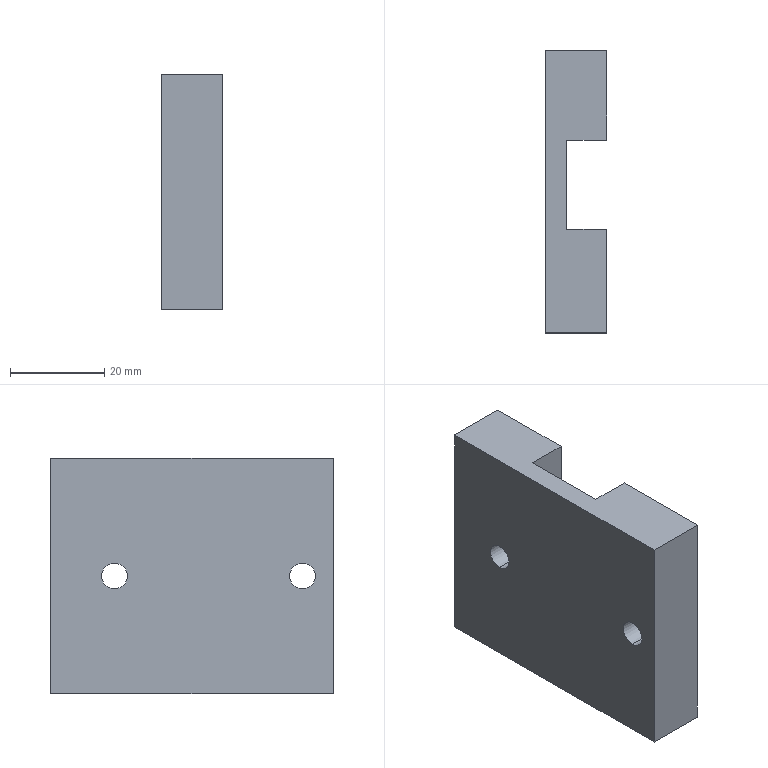Part | STEP file | PN_0039 | 1 solid | 20 faces | box 13 x 60 x 50 mm | volume 29683 mm3 | plane 12 | cylinder 8 | commonest cylinder face diameters 5.5 x4 10 x4
STEP:
#1=CARTESIAN_POINT('',(0.,0.,0.));
#2=DIRECTION('',(0.,0.,1.));
#3=DIRECTION('',(1.,0.,0.));
#4=AXIS2_PLACEMENT_3D('',#1,#2,#3);
#5=CARTESIAN_POINT('',(19.5,80.,-2.75));
#6=VERTEX_POINT('',#5);
#7=CARTESIAN_POINT('',(26.8,80.,-2.75));
#8=VERTEX_POINT('',#7);
#9=CARTESIAN_POINT('',(23.4,80.,-2.75));
#10=DIRECTION('',(1.,0.,0.));
#11=VECTOR('',#10,1.);
#12=LINE('',#9,#11);
#13=CARTESIAN_POINT('',(23.4,80.,0.));
#14=DIRECTION('',(1.,0.,0.));
#15=DIRECTION('',(0.,0.,-1.));
#16=AXIS2_PLACEMENT_3D('',#13,#14,#15);
#17=CYLINDRICAL_SURFACE('',#16,2.75);
#18=CARTESIAN_POINT('',(6.283,0.));
#19=DIRECTION('',(0.,1.));
#20=VECTOR('',#19,1.);
#21=LINE('',#18,#20);
#22=(GEOMETRIC_REPRESENTATION_CONTEXT(2)PARAMETRIC_REPRESENTATION_CONTEXT()REPRESENTATION_CONTEXT('',''));
#23=DEFINITIONAL_REPRESENTATION('',(#21),#22);
#24=PCURVE('',#17,#23);
#25=CARTESIAN_POINT('',(23.4,80.,0.));
#26=DIRECTION('',(1.,0.,0.));
#27=DIRECTION('',(0.,0.,-1.));
#28=AXIS2_PLACEMENT_3D('',#25,#26,#27);
#29=CYLINDRICAL_SURFACE('',#28,2.75);
#30=CARTESIAN_POINT('',(0.,0.));
#31=DIRECTION('',(0.,1.));
#32=VECTOR('',#31,1.);
#33=LINE('',#30,#32);
#34=(GEOMETRIC_REPRESENTATION_CONTEXT(2)PARAMETRIC_REPRESENTATION_CONTEXT()REPRESENTATION_CONTEXT('',''));
#35=DEFINITIONAL_REPRESENTATION('',(#33),#34);
#36=PCURVE('',#29,#35);
#37=SURFACE_CURVE('',#12,(#24,#36),.PCURVE_S1.);
#38=EDGE_CURVE('',#6,#8,#37,.T.);
#39=ORIENTED_EDGE('',*,*,#38,.T.);
#40=CARTESIAN_POINT('',(26.8,80.,2.75));
#41=VERTEX_POINT('',#40);
#42=CARTESIAN_POINT('',(26.8,80.,0.));
#43=DIRECTION('',(-1.,0.,0.));
#44=DIRECTION('',(0.,0.,-1.));
#45=AXIS2_PLACEMENT_3D('',#42,#43,#44);
#46=CIRCLE('',#45,2.75);
#47=CARTESIAN_POINT('',(6.283,3.4));
#48=DIRECTION('',(-1.,0.));
#49=VECTOR('',#48,1.);
#50=LINE('',#47,#49);
#51=(GEOMETRIC_REPRESENTATION_CONTEXT(2)PARAMETRIC_REPRESENTATION_CONTEXT()REPRESENTATION_CONTEXT('',''));
#52=DEFINITIONAL_REPRESENTATION('',(#50),#51);
#53=PCURVE('',#17,#52);
#54=CARTESIAN_POINT('',(26.8,83.875,0.));
#55=DIRECTION('',(-1.,0.,0.));
#56=DIRECTION('',(0.,0.,1.));
#57=AXIS2_PLACEMENT_3D('',#54,#55,#56);
#58=PLANE('',#57);
#59=CARTESIAN_POINT('',(0.,-3.875));
#60=DIRECTION('',(-1.,0.));
#61=AXIS2_PLACEMENT_2D('',#59,#60);
#62=CIRCLE('',#61,2.75);
#63=(GEOMETRIC_REPRESENTATION_CONTEXT(2)PARAMETRIC_REPRESENTATION_CONTEXT()REPRESENTATION_CONTEXT('',''));
#64=DEFINITIONAL_REPRESENTATION('',(#62),#63);
#65=PCURVE('',#58,#64);
#66=SURFACE_CURVE('',#46,(#53,#65),.PCURVE_S1.);
#67=EDGE_CURVE('',#8,#41,#66,.T.);
#68=ORIENTED_EDGE('',*,*,#67,.T.);
#69=CARTESIAN_POINT('',(19.5,80.,2.75));
#70=VERTEX_POINT('',#69);
#71=CARTESIAN_POINT('',(23.4,80.,2.75));
#72=DIRECTION('',(1.,0.,0.));
#73=VECTOR('',#72,1.);
#74=LINE('',#71,#73);
#75=CARTESIAN_POINT('',(3.142,0.));
#76=DIRECTION('',(0.,1.));
#77=VECTOR('',#76,1.);
#78=LINE('',#75,#77);
#79=(GEOMETRIC_REPRESENTATION_CONTEXT(2)PARAMETRIC_REPRESENTATION_CONTEXT()REPRESENTATION_CONTEXT('',''));
#80=DEFINITIONAL_REPRESENTATION('',(#78),#79);
#81=PCURVE('',#17,#80);
#82=CARTESIAN_POINT('',(3.142,0.));
#83=DIRECTION('',(0.,1.));
#84=VECTOR('',#83,1.);
#85=LINE('',#82,#84);
#86=(GEOMETRIC_REPRESENTATION_CONTEXT(2)PARAMETRIC_REPRESENTATION_CONTEXT()REPRESENTATION_CONTEXT('',''));
#87=DEFINITIONAL_REPRESENTATION('',(#85),#86);
#88=PCURVE('',#29,#87);
#89=SURFACE_CURVE('',#74,(#81,#88),.PCURVE_S1.);
#90=EDGE_CURVE('',#70,#41,#89,.T.);
#91=ORIENTED_EDGE('',*,*,#90,.F.);
#92=CARTESIAN_POINT('',(19.5,80.,0.));
#93=DIRECTION('',(-1.,0.,0.));
#94=DIRECTION('',(0.,0.,1.));
#95=AXIS2_PLACEMENT_3D('',#92,#93,#94);
#96=CIRCLE('',#95,2.75);
#97=CARTESIAN_POINT('',(9.425,-3.9));
#98=DIRECTION('',(-1.,0.));
#99=VECTOR('',#98,1.);
#100=LINE('',#97,#99);
#101=(GEOMETRIC_REPRESENTATION_CONTEXT(2)PARAMETRIC_REPRESENTATION_CONTEXT()REPRESENTATION_CONTEXT('',''));
#102=DEFINITIONAL_REPRESENTATION('',(#100),#101);
#103=PCURVE('',#17,#102);
#104=CARTESIAN_POINT('',(19.5,33.5,-25.));
#105=DIRECTION('',(-1.,0.,0.));
#106=DIRECTION('',(0.,0.,1.));
#107=AXIS2_PLACEMENT_3D('',#104,#105,#106);
#108=PLANE('',#107);
#109=CARTESIAN_POINT('',(25.,46.5));
#110=DIRECTION('',(1.,0.));
#111=AXIS2_PLACEMENT_2D('',#109,#110);
#112=CIRCLE('',#111,2.75);
#113=(GEOMETRIC_REPRESENTATION_CONTEXT(2)PARAMETRIC_REPRESENTATION_CONTEXT()REPRESENTATION_CONTEXT('',''));
#114=DEFINITIONAL_REPRESENTATION('',(#112),#113);
#115=PCURVE('',#108,#114);
#116=SURFACE_CURVE('',#96,(#103,#115),.PCURVE_S1.);
#117=EDGE_CURVE('',#6,#70,#116,.T.);
#118=ORIENTED_EDGE('',*,*,#117,.F.);
#119=EDGE_LOOP('',(#39,#68,#91,#118));
#120=FACE_BOUND('',#119,.F.);
#121=ADVANCED_FACE('',(#120),#17,.F.);
#122=CARTESIAN_POINT('',(19.5,40.,-2.75));
#123=VERTEX_POINT('',#122);
#124=CARTESIAN_POINT('',(26.8,40.,-2.75));
#125=VERTEX_POINT('',#124);
#126=CARTESIAN_POINT('',(23.4,40.,-2.75));
#127=DIRECTION('',(1.,0.,0.));
#128=VECTOR('',#127,1.);
#129=LINE('',#126,#128);
#130=CARTESIAN_POINT('',(23.4,40.,0.));
#131=DIRECTION('',(1.,0.,0.));
#132=DIRECTION('',(0.,0.,-1.));
#133=AXIS2_PLACEMENT_3D('',#130,#131,#132);
#134=CYLINDRICAL_SURFACE('',#133,2.75);
#135=CARTESIAN_POINT('',(6.283,0.));
#136=DIRECTION('',(0.,1.));
#137=VECTOR('',#136,1.);
#138=LINE('',#135,#137);
#139=(GEOMETRIC_REPRESENTATION_CONTEXT(2)PARAMETRIC_REPRESENTATION_CONTEXT()REPRESENTATION_CONTEXT('',''));
#140=DEFINITIONAL_REPRESENTATION('',(#138),#139);
#141=PCURVE('',#134,#140);
#142=CARTESIAN_POINT('',(23.4,40.,0.));
#143=DIRECTION('',(1.,0.,0.));
#144=DIRECTION('',(0.,0.,-1.));
#145=AXIS2_PLACEMENT_3D('',#142,#143,#144);
#146=CYLINDRICAL_SURFACE('',#145,2.75);
#147=CARTESIAN_POINT('',(0.,0.));
#148=DIRECTION('',(0.,1.));
#149=VECTOR('',#148,1.);
#150=LINE('',#147,#149);
#151=(GEOMETRIC_REPRESENTATION_CONTEXT(2)PARAMETRIC_REPRESENTATION_CONTEXT()REPRESENTATION_CONTEXT('',''));
#152=DEFINITIONAL_REPRESENTATION('',(#150),#151);
#153=PCURVE('',#146,#152);
#154=SURFACE_CURVE('',#129,(#141,#153),.PCURVE_S1.);
#155=EDGE_CURVE('',#123,#125,#154,.T.);
#156=ORIENTED_EDGE('',*,*,#155,.T.);
#157=CARTESIAN_POINT('',(26.8,40.,2.75));
#158=VERTEX_POINT('',#157);
#159=CARTESIAN_POINT('',(26.8,40.,0.));
#160=DIRECTION('',(-1.,0.,0.));
#161=DIRECTION('',(0.,0.,-1.));
#162=AXIS2_PLACEMENT_3D('',#159,#160,#161);
#163=CIRCLE('',#162,2.75);
#164=CARTESIAN_POINT('',(6.283,3.4));
#165=DIRECTION('',(-1.,0.));
#166=VECTOR('',#165,1.);
#167=LINE('',#164,#166);
#168=(GEOMETRIC_REPRESENTATION_CONTEXT(2)PARAMETRIC_REPRESENTATION_CONTEXT()REPRESENTATION_CONTEXT('',''));
#169=DEFINITIONAL_REPRESENTATION('',(#167),#168);
#170=PCURVE('',#134,#169);
#171=CARTESIAN_POINT('',(26.8,43.875,0.));
#172=DIRECTION('',(-1.,0.,0.));
#173=DIRECTION('',(0.,0.,1.));
#174=AXIS2_PLACEMENT_3D('',#171,#172,#173);
#175=PLANE('',#174);
#176=CARTESIAN_POINT('',(0.,-3.875));
#177=DIRECTION('',(-1.,0.));
#178=AXIS2_PLACEMENT_2D('',#176,#177);
#179=CIRCLE('',#178,2.75);
#180=(GEOMETRIC_REPRESENTATION_CONTEXT(2)PARAMETRIC_REPRESENTATION_CONTEXT()REPRESENTATION_CONTEXT('',''));
#181=DEFINITIONAL_REPRESENTATION('',(#179),#180);
#182=PCURVE('',#175,#181);
#183=SURFACE_CURVE('',#163,(#170,#182),.PCURVE_S1.);
#184=EDGE_CURVE('',#125,#158,#183,.T.);
#185=ORIENTED_EDGE('',*,*,#184,.T.);
#186=CARTESIAN_POINT('',(19.5,40.,2.75));
#187=VERTEX_POINT('',#186);
#188=CARTESIAN_POINT('',(23.4,40.,2.75));
#189=DIRECTION('',(1.,0.,0.));
#190=VECTOR('',#189,1.);
#191=LINE('',#188,#190);
#192=CARTESIAN_POINT('',(3.142,0.));
#193=DIRECTION('',(0.,1.));
#194=VECTOR('',#193,1.);
#195=LINE('',#192,#194);
#196=(GEOMETRIC_REPRESENTATION_CONTEXT(2)PARAMETRIC_REPRESENTATION_CONTEXT()REPRESENTATION_CONTEXT('',''));
#197=DEFINITIONAL_REPRESENTATION('',(#195),#196);
#198=PCURVE('',#134,#197);
#199=CARTESIAN_POINT('',(3.142,0.));
#200=DIRECTION('',(0.,1.));
#201=VECTOR('',#200,1.);
#202=LINE('',#199,#201);
#203=(GEOMETRIC_REPRESENTATION_CONTEXT(2)PARAMETRIC_REPRESENTATION_CONTEXT()REPRESENTATION_CONTEXT('',''));
#204=DEFINITIONAL_REPRESENTATION('',(#202),#203);
#205=PCURVE('',#146,#204);
#206=SURFACE_CURVE('',#191,(#198,#205),.PCURVE_S1.);
#207=EDGE_CURVE('',#187,#158,#206,.T.);
#208=ORIENTED_EDGE('',*,*,#207,.F.);
#209=CARTESIAN_POINT('',(19.5,40.,0.));
#210=DIRECTION('',(-1.,0.,0.));
#211=DIRECTION('',(0.,0.,1.));
#212=AXIS2_PLACEMENT_3D('',#209,#210,#211);
#213=CIRCLE('',#212,2.75);
#214=CARTESIAN_POINT('',(9.425,-3.9));
#215=DIRECTION('',(-1.,0.));
#216=VECTOR('',#215,1.);
#217=LINE('',#214,#216);
#218=(GEOMETRIC_REPRESENTATION_CONTEXT(2)PARAMETRIC_REPRESENTATION_CONTEXT()REPRESENTATION_CONTEXT('',''));
#219=DEFINITIONAL_REPRESENTATION('',(#217),#218);
#220=PCURVE('',#134,#219);
#221=CARTESIAN_POINT('',(25.,6.5));
#222=DIRECTION('',(1.,0.));
#223=AXIS2_PLACEMENT_2D('',#221,#222);
#224=CIRCLE('',#223,2.75);
#225=(GEOMETRIC_REPRESENTATION_CONTEXT(2)PARAMETRIC_REPRESENTATION_CONTEXT()REPRESENTATION_CONTEXT('',''));
#226=DEFINITIONAL_REPRESENTATION('',(#224),#225);
#227=PCURVE('',#108,#226);
#228=SURFACE_CURVE('',#213,(#220,#227),.PCURVE_S1.);
#229=EDGE_CURVE('',#123,#187,#228,.T.);
#230=ORIENTED_EDGE('',*,*,#229,.F.);
#231=EDGE_LOOP('',(#156,#185,#208,#230));
#232=FACE_BOUND('',#231,.F.);
#233=ADVANCED_FACE('',(#232),#134,.F.);
#234=CARTESIAN_POINT('',(26.8,80.,-5.));
#235=VERTEX_POINT('',#234);
#236=CARTESIAN_POINT('',(32.5,80.,-5.));
#237=VERTEX_POINT('',#236);
#238=CARTESIAN_POINT('',(29.65,80.,-5.));
#239=DIRECTION('',(1.,0.,0.));
#240=VECTOR('',#239,1.);
#241=LINE('',#238,#240);
#242=CARTESIAN_POINT('',(29.65,80.,0.));
#243=DIRECTION('',(1.,0.,0.));
#244=DIRECTION('',(0.,0.,-1.));
#245=AXIS2_PLACEMENT_3D('',#242,#243,#244);
#246=CYLINDRICAL_SURFACE('',#245,5.);
#247=CARTESIAN_POINT('',(6.283,0.));
#248=DIRECTION('',(0.,1.));
#249=VECTOR('',#248,1.);
#250=LINE('',#247,#249);
#251=(GEOMETRIC_REPRESENTATION_CONTEXT(2)PARAMETRIC_REPRESENTATION_CONTEXT()REPRESENTATION_CONTEXT('',''));
#252=DEFINITIONAL_REPRESENTATION('',(#250),#251);
#253=PCURVE('',#246,#252);
#254=CARTESIAN_POINT('',(29.65,80.,0.));
#255=DIRECTION('',(1.,0.,0.));
#256=DIRECTION('',(0.,0.,-1.));
#257=AXIS2_PLACEMENT_3D('',#254,#255,#256);
#258=CYLINDRICAL_SURFACE('',#257,5.);
#259=CARTESIAN_POINT('',(0.,0.));
#260=DIRECTION('',(0.,1.));
#261=VECTOR('',#260,1.);
#262=LINE('',#259,#261);
#263=(GEOMETRIC_REPRESENTATION_CONTEXT(2)PARAMETRIC_REPRESENTATION_CONTEXT()REPRESENTATION_CONTEXT('',''));
#264=DEFINITIONAL_REPRESENTATION('',(#262),#263);
#265=PCURVE('',#258,#264);
#266=SURFACE_CURVE('',#241,(#253,#265),.PCURVE_S1.);
#267=EDGE_CURVE('',#235,#237,#266,.T.);
#268=ORIENTED_EDGE('',*,*,#267,.T.);
#269=CARTESIAN_POINT('',(32.5,80.,5.));
#270=VERTEX_POINT('',#269);
#271=CARTESIAN_POINT('',(32.5,80.,0.));
#272=DIRECTION('',(-1.,0.,0.));
#273=DIRECTION('',(0.,0.,-1.));
#274=AXIS2_PLACEMENT_3D('',#271,#272,#273);
#275=CIRCLE('',#274,5.);
#276=CARTESIAN_POINT('',(6.283,2.85));
#277=DIRECTION('',(-1.,0.));
#278=VECTOR('',#277,1.);
#279=LINE('',#276,#278);
#280=(GEOMETRIC_REPRESENTATION_CONTEXT(2)PARAMETRIC_REPRESENTATION_CONTEXT()REPRESENTATION_CONTEXT('',''));
#281=DEFINITIONAL_REPRESENTATION('',(#279),#280);
#282=PCURVE('',#246,#281);
#283=CARTESIAN_POINT('',(32.5,74.5,25.));
#284=DIRECTION('',(1.,0.,0.));
#285=DIRECTION('',(0.,0.,-1.));
#286=AXIS2_PLACEMENT_3D('',#283,#284,#285);
#287=PLANE('',#286);
#288=CARTESIAN_POINT('',(30.,5.5));
#289=CARTESIAN_POINT('',(30.,-3.16));
#290=CARTESIAN_POINT('',(22.5,1.17));
#291=CARTESIAN_POINT('',(15.,5.5));
#292=CARTESIAN_POINT('',(22.5,9.83));
#293=CARTESIAN_POINT('',(30.,14.16));
#294=CARTESIAN_POINT('',(30.,5.5));
#295=(BOUNDED_CURVE()B_SPLINE_CURVE(2,(#288,#289,#290,#291,#292,#293,#294),.UNSPECIFIED.,.T.,.F.)B_SPLINE_CURVE_WITH_KNOTS((1,2,2,2,2,1),(-2.094,0.,2.094,4.189,6.283,8.378),.UNSPECIFIED.)CURVE()GEOMETRIC_REPRESENTATION_ITEM()RATIONAL_B_SPLINE_CURVE((1.,0.5,1.,0.5,1.,0.5,1.))REPRESENTATION_ITEM(''));
#296=(GEOMETRIC_REPRESENTATION_CONTEXT(2)PARAMETRIC_REPRESENTATION_CONTEXT()REPRESENTATION_CONTEXT('',''));
#297=DEFINITIONAL_REPRESENTATION('',(#295),#296);
#298=PCURVE('',#287,#297);
#299=SURFACE_CURVE('',#275,(#282,#298),.PCURVE_S1.);
#300=EDGE_CURVE('',#237,#270,#299,.T.);
#301=ORIENTED_EDGE('',*,*,#300,.T.);
#302=CARTESIAN_POINT('',(26.8,80.,5.));
#303=VERTEX_POINT('',#302);
#304=CARTESIAN_POINT('',(29.65,80.,5.));
#305=DIRECTION('',(1.,0.,0.));
#306=VECTOR('',#305,1.);
#307=LINE('',#304,#306);
#308=CARTESIAN_POINT('',(3.142,0.));
#309=DIRECTION('',(0.,1.));
#310=VECTOR('',#309,1.);
#311=LINE('',#308,#310);
#312=(GEOMETRIC_REPRESENTATION_CONTEXT(2)PARAMETRIC_REPRESENTATION_CONTEXT()REPRESENTATION_CONTEXT('',''));
#313=DEFINITIONAL_REPRESENTATION('',(#311),#312);
#314=PCURVE('',#246,#313);
#315=CARTESIAN_POINT('',(3.142,0.));
#316=DIRECTION('',(0.,1.));
#317=VECTOR('',#316,1.);
#318=LINE('',#315,#317);
#319=(GEOMETRIC_REPRESENTATION_CONTEXT(2)PARAMETRIC_REPRESENTATION_CONTEXT()REPRESENTATION_CONTEXT('',''));
#320=DEFINITIONAL_REPRESENTATION('',(#318),#319);
#321=PCURVE('',#258,#320);
#322=SURFACE_CURVE('',#307,(#314,#321),.PCURVE_S1.);
#323=EDGE_CURVE('',#303,#270,#322,.T.);
#324=ORIENTED_EDGE('',*,*,#323,.F.);
#325=CARTESIAN_POINT('',(26.8,80.,0.));
#326=DIRECTION('',(-1.,0.,0.));
#327=DIRECTION('',(0.,0.,-1.));
#328=AXIS2_PLACEMENT_3D('',#325,#326,#327);
#329=CIRCLE('',#328,5.);
#330=CARTESIAN_POINT('',(6.283,-2.85));
#331=DIRECTION('',(-1.,0.));
#332=VECTOR('',#331,1.);
#333=LINE('',#330,#332);
#334=(GEOMETRIC_REPRESENTATION_CONTEXT(2)PARAMETRIC_REPRESENTATION_CONTEXT()REPRESENTATION_CONTEXT('',''));
#335=DEFINITIONAL_REPRESENTATION('',(#333),#334);
#336=PCURVE('',#246,#335);
#337=CARTESIAN_POINT('',(0.,-3.875));
#338=DIRECTION('',(-1.,0.));
#339=AXIS2_PLACEMENT_2D('',#337,#338);
#340=CIRCLE('',#339,5.);
#341=(GEOMETRIC_REPRESENTATION_CONTEXT(2)PARAMETRIC_REPRESENTATION_CONTEXT()REPRESENTATION_CONTEXT('',''));
#342=DEFINITIONAL_REPRESENTATION('',(#340),#341);
#343=PCURVE('',#58,#342);
#344=SURFACE_CURVE('',#329,(#336,#343),.PCURVE_S1.);
#345=EDGE_CURVE('',#235,#303,#344,.T.);
#346=ORIENTED_EDGE('',*,*,#345,.F.);
#347=EDGE_LOOP('',(#268,#301,#324,#346));
#348=FACE_BOUND('',#347,.F.);
#349=ADVANCED_FACE('',(#348),#246,.F.);
#350=CARTESIAN_POINT('',(26.8,40.,-5.));
#351=VERTEX_POINT('',#350);
#352=CARTESIAN_POINT('',(32.5,40.,-5.));
#353=VERTEX_POINT('',#352);
#354=CARTESIAN_POINT('',(29.65,40.,-5.));
#355=DIRECTION('',(1.,0.,0.));
#356=VECTOR('',#355,1.);
#357=LINE('',#354,#356);
#358=CARTESIAN_POINT('',(29.65,40.,0.));
#359=DIRECTION('',(1.,0.,0.));
#360=DIRECTION('',(0.,0.,-1.));
#361=AXIS2_PLACEMENT_3D('',#358,#359,#360);
#362=CYLINDRICAL_SURFACE('',#361,5.);
#363=CARTESIAN_POINT('',(6.283,0.));
#364=DIRECTION('',(0.,1.));
#365=VECTOR('',#364,1.);
#366=LINE('',#363,#365);
#367=(GEOMETRIC_REPRESENTATION_CONTEXT(2)PARAMETRIC_REPRESENTATION_CONTEXT()REPRESENTATION_CONTEXT('',''));
#368=DEFINITIONAL_REPRESENTATION('',(#366),#367);
#369=PCURVE('',#362,#368);
#370=CARTESIAN_POINT('',(29.65,40.,0.));
#371=DIRECTION('',(1.,0.,0.));
#372=DIRECTION('',(0.,0.,-1.));
#373=AXIS2_PLACEMENT_3D('',#370,#371,#372);
#374=CYLINDRICAL_SURFACE('',#373,5.);
#375=CARTESIAN_POINT('',(0.,0.));
#376=DIRECTION('',(0.,1.));
#377=VECTOR('',#376,1.);
#378=LINE('',#375,#377);
#379=(GEOMETRIC_REPRESENTATION_CONTEXT(2)PARAMETRIC_REPRESENTATION_CONTEXT()REPRESENTATION_CONTEXT('',''));
#380=DEFINITIONAL_REPRESENTATION('',(#378),#379);
#381=PCURVE('',#374,#380);
#382=SURFACE_CURVE('',#357,(#369,#381),.PCURVE_S1.);
#383=EDGE_CURVE('',#351,#353,#382,.T.);
#384=ORIENTED_EDGE('',*,*,#383,.T.);
#385=CARTESIAN_POINT('',(32.5,40.,5.));
#386=VERTEX_POINT('',#385);
#387=CARTESIAN_POINT('',(32.5,40.,0.));
#388=DIRECTION('',(-1.,0.,0.));
#389=DIRECTION('',(0.,0.,-1.));
#390=AXIS2_PLACEMENT_3D('',#387,#388,#389);
#391=CIRCLE('',#390,5.);
#392=CARTESIAN_POINT('',(6.283,2.85));
#393=DIRECTION('',(-1.,0.));
#394=VECTOR('',#393,1.);
#395=LINE('',#392,#394);
#396=(GEOMETRIC_REPRESENTATION_CONTEXT(2)PARAMETRIC_REPRESENTATION_CONTEXT()REPRESENTATION_CONTEXT('',''));
#397=DEFINITIONAL_REPRESENTATION('',(#395),#396);
#398=PCURVE('',#362,#397);
#399=CARTESIAN_POINT('',(32.5,33.5,25.));
#400=DIRECTION('',(1.,0.,0.));
#401=DIRECTION('',(0.,0.,-1.));
#402=AXIS2_PLACEMENT_3D('',#399,#400,#401);
#403=PLANE('',#402);
#404=CARTESIAN_POINT('',(30.,6.5));
#405=CARTESIAN_POINT('',(30.,-2.16));
#406=CARTESIAN_POINT('',(22.5,2.17));
#407=CARTESIAN_POINT('',(15.,6.5));
#408=CARTESIAN_POINT('',(22.5,10.83));
#409=CARTESIAN_POINT('',(30.,15.16));
#410=CARTESIAN_POINT('',(30.,6.5));
#411=(BOUNDED_CURVE()B_SPLINE_CURVE(2,(#404,#405,#406,#407,#408,#409,#410),.UNSPECIFIED.,.T.,.F.)B_SPLINE_CURVE_WITH_KNOTS((1,2,2,2,2,1),(-2.094,0.,2.094,4.189,6.283,8.378),.UNSPECIFIED.)CURVE()GEOMETRIC_REPRESENTATION_ITEM()RATIONAL_B_SPLINE_CURVE((1.,0.5,1.,0.5,1.,0.5,1.))REPRESENTATION_ITEM(''));
#412=(GEOMETRIC_REPRESENTATION_CONTEXT(2)PARAMETRIC_REPRESENTATION_CONTEXT()REPRESENTATION_CONTEXT('',''));
#413=DEFINITIONAL_REPRESENTATION('',(#411),#412);
#414=PCURVE('',#403,#413);
#415=SURFACE_CURVE('',#391,(#398,#414),.PCURVE_S1.);
#416=EDGE_CURVE('',#353,#386,#415,.T.);
#417=ORIENTED_EDGE('',*,*,#416,.T.);
#418=CARTESIAN_POINT('',(26.8,40.,5.));
#419=VERTEX_POINT('',#418);
#420=CARTESIAN_POINT('',(29.65,40.,5.));
#421=DIRECTION('',(1.,0.,0.));
#422=VECTOR('',#421,1.);
#423=LINE('',#420,#422);
#424=CARTESIAN_POINT('',(3.142,0.));
#425=DIRECTION('',(0.,1.));
#426=VECTOR('',#425,1.);
#427=LINE('',#424,#426);
#428=(GEOMETRIC_REPRESENTATION_CONTEXT(2)PARAMETRIC_REPRESENTATION_CONTEXT()REPRESENTATION_CONTEXT('',''));
#429=DEFINITIONAL_REPRESENTATION('',(#427),#428);
#430=PCURVE('',#362,#429);
#431=CARTESIAN_POINT('',(3.142,0.));
#432=DIRECTION('',(0.,1.));
#433=VECTOR('',#432,1.);
#434=LINE('',#431,#433);
#435=(GEOMETRIC_REPRESENTATION_CONTEXT(2)PARAMETRIC_REPRESENTATION_CONTEXT()REPRESENTATION_CONTEXT('',''));
#436=DEFINITIONAL_REPRESENTATION('',(#434),#435);
#437=PCURVE('',#374,#436);
#438=SURFACE_CURVE('',#423,(#430,#437),.PCURVE_S1.);
#439=EDGE_CURVE('',#419,#386,#438,.T.);
#440=ORIENTED_EDGE('',*,*,#439,.F.);
#441=CARTESIAN_POINT('',(26.8,40.,0.));
#442=DIRECTION('',(-1.,0.,0.));
#443=DIRECTION('',(0.,0.,-1.));
#444=AXIS2_PLACEMENT_3D('',#441,#442,#443);
#445=CIRCLE('',#444,5.);
#446=CARTESIAN_POINT('',(6.283,-2.85));
#447=DIRECTION('',(-1.,0.));
#448=VECTOR('',#447,1.);
#449=LINE('',#446,#448);
#450=(GEOMETRIC_REPRESENTATION_CONTEXT(2)PARAMETRIC_REPRESENTATION_CONTEXT()REPRESENTATION_CONTEXT('',''));
#451=DEFINITIONAL_REPRESENTATION('',(#449),#450);
#452=PCURVE('',#362,#451);
#453=CARTESIAN_POINT('',(0.,-3.875));
#454=DIRECTION('',(-1.,0.));
#455=AXIS2_PLACEMENT_2D('',#453,#454);
#456=CIRCLE('',#455,5.);
#457=(GEOMETRIC_REPRESENTATION_CONTEXT(2)PARAMETRIC_REPRESENTATION_CONTEXT()REPRESENTATION_CONTEXT('',''));
#458=DEFINITIONAL_REPRESENTATION('',(#456),#457);
#459=PCURVE('',#175,#458);
#460=SURFACE_CURVE('',#445,(#452,#459),.PCURVE_S1.);
#461=EDGE_CURVE('',#351,#419,#460,.T.);
#462=ORIENTED_EDGE('',*,*,#461,.F.);
#463=EDGE_LOOP('',(#384,#417,#440,#462));
#464=FACE_BOUND('',#463,.F.);
#465=ADVANCED_FACE('',(#464),#362,.F.);
#466=CARTESIAN_POINT('',(19.5,93.5,25.));
#467=VERTEX_POINT('',#466);
#468=CARTESIAN_POINT('',(32.5,93.5,25.));
#469=VERTEX_POINT('',#468);
#470=CARTESIAN_POINT('',(32.5,93.5,25.));
#471=DIRECTION('',(1.,0.,0.));
#472=VECTOR('',#471,1.);
#473=LINE('',#470,#472);
#474=CARTESIAN_POINT('',(32.5,93.5,25.));
#475=DIRECTION('',(0.,1.,0.));
#476=DIRECTION('',(0.,0.,1.));
#477=AXIS2_PLACEMENT_3D('',#474,#475,#476);
#478=PLANE('',#477);
#479=CARTESIAN_POINT('',(0.,0.));
#480=DIRECTION('',(0.,1.));
#481=VECTOR('',#480,1.);
#482=LINE('',#479,#481);
#483=(GEOMETRIC_REPRESENTATION_CONTEXT(2)PARAMETRIC_REPRESENTATION_CONTEXT()REPRESENTATION_CONTEXT('',''));
#484=DEFINITIONAL_REPRESENTATION('',(#482),#483);
#485=PCURVE('',#478,#484);
#486=CARTESIAN_POINT('',(32.5,33.5,25.));
#487=DIRECTION('',(0.,0.,1.));
#488=DIRECTION('',(1.,0.,0.));
#489=AXIS2_PLACEMENT_3D('',#486,#487,#488);
#490=PLANE('',#489);
#491=CARTESIAN_POINT('',(0.,60.));
#492=DIRECTION('',(1.,0.));
#493=VECTOR('',#492,1.);
#494=LINE('',#491,#493);
#495=(GEOMETRIC_REPRESENTATION_CONTEXT(2)PARAMETRIC_REPRESENTATION_CONTEXT()REPRESENTATION_CONTEXT('',''));
#496=DEFINITIONAL_REPRESENTATION('',(#494),#495);
#497=PCURVE('',#490,#496);
#498=SURFACE_CURVE('',#473,(#485,#497),.PCURVE_S1.);
#499=EDGE_CURVE('',#467,#469,#498,.T.);
#500=ORIENTED_EDGE('',*,*,#499,.T.);
#501=CARTESIAN_POINT('',(32.5,93.5,-25.));
#502=VERTEX_POINT('',#501);
#503=CARTESIAN_POINT('',(32.5,93.5,25.));
#504=DIRECTION('',(0.,0.,-1.));
#505=VECTOR('',#504,1.);
#506=LINE('',#503,#505);
#507=CARTESIAN_POINT('',(0.,0.));
#508=DIRECTION('',(-1.,0.));
#509=VECTOR('',#508,1.);
#510=LINE('',#507,#509);
#511=(GEOMETRIC_REPRESENTATION_CONTEXT(2)PARAMETRIC_REPRESENTATION_CONTEXT()REPRESENTATION_CONTEXT('',''));
#512=DEFINITIONAL_REPRESENTATION('',(#510),#511);
#513=PCURVE('',#478,#512);
#514=CARTESIAN_POINT('',(0.,19.));
#515=DIRECTION('',(1.,0.));
#516=VECTOR('',#515,1.);
#517=LINE('',#514,#516);
#518=(GEOMETRIC_REPRESENTATION_CONTEXT(2)PARAMETRIC_REPRESENTATION_CONTEXT()REPRESENTATION_CONTEXT('',''));
#519=DEFINITIONAL_REPRESENTATION('',(#517),#518);
#520=PCURVE('',#287,#519);
#521=SURFACE_CURVE('',#506,(#513,#520),.PCURVE_S1.);
#522=EDGE_CURVE('',#469,#502,#521,.T.);
#523=ORIENTED_EDGE('',*,*,#522,.T.);
#524=CARTESIAN_POINT('',(19.5,93.5,-25.));
#525=VERTEX_POINT('',#524);
#526=CARTESIAN_POINT('',(32.5,93.5,-25.));
#527=DIRECTION('',(-1.,0.,0.));
#528=VECTOR('',#527,1.);
#529=LINE('',#526,#528);
#530=CARTESIAN_POINT('',(-50.,0.));
#531=DIRECTION('',(0.,-1.));
#532=VECTOR('',#531,1.);
#533=LINE('',#530,#532);
#534=(GEOMETRIC_REPRESENTATION_CONTEXT(2)PARAMETRIC_REPRESENTATION_CONTEXT()REPRESENTATION_CONTEXT('',''));
#535=DEFINITIONAL_REPRESENTATION('',(#533),#534);
#536=PCURVE('',#478,#535);
#537=CARTESIAN_POINT('',(32.5,33.5,-25.));
#538=DIRECTION('',(0.,0.,1.));
#539=DIRECTION('',(1.,0.,0.));
#540=AXIS2_PLACEMENT_3D('',#537,#538,#539);
#541=PLANE('',#540);
#542=CARTESIAN_POINT('',(0.,60.));
#543=DIRECTION('',(-1.,0.));
#544=VECTOR('',#543,1.);
#545=LINE('',#542,#544);
#546=(GEOMETRIC_REPRESENTATION_CONTEXT(2)PARAMETRIC_REPRESENTATION_CONTEXT()REPRESENTATION_CONTEXT('',''));
#547=DEFINITIONAL_REPRESENTATION('',(#545),#546);
#548=PCURVE('',#541,#547);
#549=SURFACE_CURVE('',#529,(#536,#548),.PCURVE_S1.);
#550=EDGE_CURVE('',#502,#525,#549,.T.);
#551=ORIENTED_EDGE('',*,*,#550,.T.);
#552=CARTESIAN_POINT('',(19.5,93.5,-25.));
#553=DIRECTION('',(0.,0.,-1.));
#554=VECTOR('',#553,1.);
#555=LINE('',#552,#554);
#556=CARTESIAN_POINT('',(-50.,-13.));
#557=DIRECTION('',(-1.,0.));
#558=VECTOR('',#557,1.);
#559=LINE('',#556,#558);
#560=(GEOMETRIC_REPRESENTATION_CONTEXT(2)PARAMETRIC_REPRESENTATION_CONTEXT()REPRESENTATION_CONTEXT('',''));
#561=DEFINITIONAL_REPRESENTATION('',(#559),#560);
#562=PCURVE('',#478,#561);
#563=CARTESIAN_POINT('',(0.,60.));
#564=DIRECTION('',(-1.,0.));
#565=VECTOR('',#564,1.);
#566=LINE('',#563,#565);
#567=(GEOMETRIC_REPRESENTATION_CONTEXT(2)PARAMETRIC_REPRESENTATION_CONTEXT()REPRESENTATION_CONTEXT('',''));
#568=DEFINITIONAL_REPRESENTATION('',(#566),#567);
#569=PCURVE('',#108,#568);
#570=SURFACE_CURVE('',#555,(#562,#569),.PCURVE_S1.);
#571=EDGE_CURVE('',#467,#525,#570,.T.);
#572=ORIENTED_EDGE('',*,*,#571,.F.);
#573=EDGE_LOOP('',(#500,#523,#551,#572));
#574=FACE_BOUND('',#573,.T.);
#575=ADVANCED_FACE('',(#574),#478,.T.);
#576=ORIENTED_EDGE('',*,*,#499,.F.);
#577=CARTESIAN_POINT('',(19.5,33.5,25.));
#578=VERTEX_POINT('',#577);
#579=CARTESIAN_POINT('',(19.5,93.5,25.));
#580=DIRECTION('',(0.,1.,0.));
#581=VECTOR('',#580,1.);
#582=LINE('',#579,#581);
#583=CARTESIAN_POINT('',(-13.,60.));
#584=DIRECTION('',(0.,1.));
#585=VECTOR('',#584,1.);
#586=LINE('',#583,#585);
#587=(GEOMETRIC_REPRESENTATION_CONTEXT(2)PARAMETRIC_REPRESENTATION_CONTEXT()REPRESENTATION_CONTEXT('',''));
#588=DEFINITIONAL_REPRESENTATION('',(#586),#587);
#589=PCURVE('',#490,#588);
#590=CARTESIAN_POINT('',(50.,60.));
#591=DIRECTION('',(0.,1.));
#592=VECTOR('',#591,1.);
#593=LINE('',#590,#592);
#594=(GEOMETRIC_REPRESENTATION_CONTEXT(2)PARAMETRIC_REPRESENTATION_CONTEXT()REPRESENTATION_CONTEXT('',''));
#595=DEFINITIONAL_REPRESENTATION('',(#593),#594);
#596=PCURVE('',#108,#595);
#597=SURFACE_CURVE('',#582,(#589,#596),.PCURVE_S1.);
#598=EDGE_CURVE('',#578,#467,#597,.T.);
#599=ORIENTED_EDGE('',*,*,#598,.F.);
#600=CARTESIAN_POINT('',(32.5,33.5,25.));
#601=VERTEX_POINT('',#600);
#602=CARTESIAN_POINT('',(32.5,33.5,25.));
#603=DIRECTION('',(1.,0.,0.));
#604=VECTOR('',#603,1.);
#605=LINE('',#602,#604);
#606=CARTESIAN_POINT('',(0.,0.));
#607=DIRECTION('',(1.,0.));
#608=VECTOR('',#607,1.);
#609=LINE('',#606,#608);
#610=(GEOMETRIC_REPRESENTATION_CONTEXT(2)PARAMETRIC_REPRESENTATION_CONTEXT()REPRESENTATION_CONTEXT('',''));
#611=DEFINITIONAL_REPRESENTATION('',(#609),#610);
#612=PCURVE('',#490,#611);
#613=CARTESIAN_POINT('',(20.,33.5,25.));
#614=DIRECTION('',(0.,-1.,0.));
#615=DIRECTION('',(0.,0.,-1.));
#616=AXIS2_PLACEMENT_3D('',#613,#614,#615);
#617=PLANE('',#616);
#618=CARTESIAN_POINT('',(0.,12.5));
#619=DIRECTION('',(0.,1.));
#620=VECTOR('',#619,1.);
#621=LINE('',#618,#620);
#622=(GEOMETRIC_REPRESENTATION_CONTEXT(2)PARAMETRIC_REPRESENTATION_CONTEXT()REPRESENTATION_CONTEXT('',''));
#623=DEFINITIONAL_REPRESENTATION('',(#621),#622);
#624=PCURVE('',#617,#623);
#625=SURFACE_CURVE('',#605,(#612,#624),.PCURVE_S1.);
#626=EDGE_CURVE('',#578,#601,#625,.T.);
#627=ORIENTED_EDGE('',*,*,#626,.T.);
#628=CARTESIAN_POINT('',(32.5,55.5,25.));
#629=VERTEX_POINT('',#628);
#630=CARTESIAN_POINT('',(32.5,33.5,25.));
#631=DIRECTION('',(0.,1.,0.));
#632=VECTOR('',#631,1.);
#633=LINE('',#630,#632);
#634=CARTESIAN_POINT('',(0.,0.));
#635=DIRECTION('',(0.,1.));
#636=VECTOR('',#635,1.);
#637=LINE('',#634,#636);
#638=(GEOMETRIC_REPRESENTATION_CONTEXT(2)PARAMETRIC_REPRESENTATION_CONTEXT()REPRESENTATION_CONTEXT('',''));
#639=DEFINITIONAL_REPRESENTATION('',(#637),#638);
#640=PCURVE('',#490,#639);
#641=CARTESIAN_POINT('',(0.,0.));
#642=DIRECTION('',(0.,1.));
#643=VECTOR('',#642,1.);
#644=LINE('',#641,#643);
#645=(GEOMETRIC_REPRESENTATION_CONTEXT(2)PARAMETRIC_REPRESENTATION_CONTEXT()REPRESENTATION_CONTEXT('',''));
#646=DEFINITIONAL_REPRESENTATION('',(#644),#645);
#647=PCURVE('',#403,#646);
#648=SURFACE_CURVE('',#633,(#640,#647),.PCURVE_S1.);
#649=EDGE_CURVE('',#601,#629,#648,.T.);
#650=ORIENTED_EDGE('',*,*,#649,.T.);
#651=CARTESIAN_POINT('',(24.,55.5,25.));
#652=VERTEX_POINT('',#651);
#653=CARTESIAN_POINT('',(32.5,55.5,25.));
#654=DIRECTION('',(-1.,0.,0.));
#655=VECTOR('',#654,1.);
#656=LINE('',#653,#655);
#657=CARTESIAN_POINT('',(0.,22.));
#658=DIRECTION('',(-1.,0.));
#659=VECTOR('',#658,1.);
#660=LINE('',#657,#659);
#661=(GEOMETRIC_REPRESENTATION_CONTEXT(2)PARAMETRIC_REPRESENTATION_CONTEXT()REPRESENTATION_CONTEXT('',''));
#662=DEFINITIONAL_REPRESENTATION('',(#660),#661);
#663=PCURVE('',#490,#662);
#664=CARTESIAN_POINT('',(32.5,55.5,25.));
#665=DIRECTION('',(0.,1.,0.));
#666=DIRECTION('',(0.,0.,1.));
#667=AXIS2_PLACEMENT_3D('',#664,#665,#666);
#668=PLANE('',#667);
#669=CARTESIAN_POINT('',(0.,0.));
#670=DIRECTION('',(0.,-1.));
#671=VECTOR('',#670,1.);
#672=LINE('',#669,#671);
#673=(GEOMETRIC_REPRESENTATION_CONTEXT(2)PARAMETRIC_REPRESENTATION_CONTEXT()REPRESENTATION_CONTEXT('',''));
#674=DEFINITIONAL_REPRESENTATION('',(#672),#673);
#675=PCURVE('',#668,#674);
#676=SURFACE_CURVE('',#656,(#663,#675),.PCURVE_S1.);
#677=EDGE_CURVE('',#629,#652,#676,.T.);
#678=ORIENTED_EDGE('',*,*,#677,.T.);
#679=CARTESIAN_POINT('',(24.,74.5,25.));
#680=VERTEX_POINT('',#679);
#681=CARTESIAN_POINT('',(24.,33.5,25.));
#682=DIRECTION('',(0.,1.,0.));
#683=VECTOR('',#682,1.);
#684=LINE('',#681,#683);
#685=CARTESIAN_POINT('',(-8.5,0.));
#686=DIRECTION('',(0.,1.));
#687=VECTOR('',#686,1.);
#688=LINE('',#685,#687);
#689=(GEOMETRIC_REPRESENTATION_CONTEXT(2)PARAMETRIC_REPRESENTATION_CONTEXT()REPRESENTATION_CONTEXT('',''));
#690=DEFINITIONAL_REPRESENTATION('',(#688),#689);
#691=PCURVE('',#490,#690);
#692=CARTESIAN_POINT('',(24.,55.5,25.));
#693=DIRECTION('',(1.,0.,0.));
#694=DIRECTION('',(0.,0.,-1.));
#695=AXIS2_PLACEMENT_3D('',#692,#693,#694);
#696=PLANE('',#695);
#697=CARTESIAN_POINT('',(0.,-22.));
#698=DIRECTION('',(0.,1.));
#699=VECTOR('',#698,1.);
#700=LINE('',#697,#699);
#701=(GEOMETRIC_REPRESENTATION_CONTEXT(2)PARAMETRIC_REPRESENTATION_CONTEXT()REPRESENTATION_CONTEXT('',''));
#702=DEFINITIONAL_REPRESENTATION('',(#700),#701);
#703=PCURVE('',#696,#702);
#704=SURFACE_CURVE('',#684,(#691,#703),.PCURVE_S1.);
#705=EDGE_CURVE('',#652,#680,#704,.T.);
#706=ORIENTED_EDGE('',*,*,#705,.T.);
#707=CARTESIAN_POINT('',(32.5,74.5,25.));
#708=VERTEX_POINT('',#707);
#709=CARTESIAN_POINT('',(32.5,74.5,25.));
#710=DIRECTION('',(1.,0.,0.));
#711=VECTOR('',#710,1.);
#712=LINE('',#709,#711);
#713=CARTESIAN_POINT('',(0.,41.));
#714=DIRECTION('',(1.,0.));
#715=VECTOR('',#714,1.);
#716=LINE('',#713,#715);
#717=(GEOMETRIC_REPRESENTATION_CONTEXT(2)PARAMETRIC_REPRESENTATION_CONTEXT()REPRESENTATION_CONTEXT('',''));
#718=DEFINITIONAL_REPRESENTATION('',(#716),#717);
#719=PCURVE('',#490,#718);
#720=CARTESIAN_POINT('',(24.,74.5,25.));
#721=DIRECTION('',(0.,-1.,0.));
#722=DIRECTION('',(0.,0.,-1.));
#723=AXIS2_PLACEMENT_3D('',#720,#721,#722);
#724=PLANE('',#723);
#725=CARTESIAN_POINT('',(0.,8.5));
#726=DIRECTION('',(0.,1.));
#727=VECTOR('',#726,1.);
#728=LINE('',#725,#727);
#729=(GEOMETRIC_REPRESENTATION_CONTEXT(2)PARAMETRIC_REPRESENTATION_CONTEXT()REPRESENTATION_CONTEXT('',''));
#730=DEFINITIONAL_REPRESENTATION('',(#728),#729);
#731=PCURVE('',#724,#730);
#732=SURFACE_CURVE('',#712,(#719,#731),.PCURVE_S1.);
#733=EDGE_CURVE('',#680,#708,#732,.T.);
#734=ORIENTED_EDGE('',*,*,#733,.T.);
#735=CARTESIAN_POINT('',(32.5,33.5,25.));
#736=DIRECTION('',(0.,1.,0.));
#737=VECTOR('',#736,1.);
#738=LINE('',#735,#737);
#739=CARTESIAN_POINT('',(0.,0.));
#740=DIRECTION('',(0.,1.));
#741=VECTOR('',#740,1.);
#742=LINE('',#739,#741);
#743=(GEOMETRIC_REPRESENTATION_CONTEXT(2)PARAMETRIC_REPRESENTATION_CONTEXT()REPRESENTATION_CONTEXT('',''));
#744=DEFINITIONAL_REPRESENTATION('',(#742),#743);
#745=PCURVE('',#490,#744);
#746=CARTESIAN_POINT('',(0.,-41.));
#747=DIRECTION('',(0.,1.));
#748=VECTOR('',#747,1.);
#749=LINE('',#746,#748);
#750=(GEOMETRIC_REPRESENTATION_CONTEXT(2)PARAMETRIC_REPRESENTATION_CONTEXT()REPRESENTATION_CONTEXT('',''));
#751=DEFINITIONAL_REPRESENTATION('',(#749),#750);
#752=PCURVE('',#287,#751);
#753=SURFACE_CURVE('',#738,(#745,#752),.PCURVE_S1.);
#754=EDGE_CURVE('',#708,#469,#753,.T.);
#755=ORIENTED_EDGE('',*,*,#754,.T.);
#756=EDGE_LOOP('',(#576,#599,#627,#650,#678,#706,#734,#755));
#757=FACE_BOUND('',#756,.T.);
#758=ADVANCED_FACE('',(#757),#490,.T.);
#759=ORIENTED_EDGE('',*,*,#626,.F.);
#760=CARTESIAN_POINT('',(19.5,33.5,-25.));
#761=VERTEX_POINT('',#760);
#762=CARTESIAN_POINT('',(19.5,33.5,-25.));
#763=DIRECTION('',(0.,0.,1.));
#764=VECTOR('',#763,1.);
#765=LINE('',#762,#764);
#766=CARTESIAN_POINT('',(50.,-0.5));
#767=DIRECTION('',(-1.,0.));
#768=VECTOR('',#767,1.);
#769=LINE('',#766,#768);
#770=(GEOMETRIC_REPRESENTATION_CONTEXT(2)PARAMETRIC_REPRESENTATION_CONTEXT()REPRESENTATION_CONTEXT('',''));
#771=DEFINITIONAL_REPRESENTATION('',(#769),#770);
#772=PCURVE('',#617,#771);
#773=CARTESIAN_POINT('',(0.,0.));
#774=DIRECTION('',(1.,0.));
#775=VECTOR('',#774,1.);
#776=LINE('',#773,#775);
#777=(GEOMETRIC_REPRESENTATION_CONTEXT(2)PARAMETRIC_REPRESENTATION_CONTEXT()REPRESENTATION_CONTEXT('',''));
#778=DEFINITIONAL_REPRESENTATION('',(#776),#777);
#779=PCURVE('',#108,#778);
#780=SURFACE_CURVE('',#765,(#772,#779),.PCURVE_S1.);
#781=EDGE_CURVE('',#761,#578,#780,.T.);
#782=ORIENTED_EDGE('',*,*,#781,.F.);
#783=CARTESIAN_POINT('',(32.5,33.5,-25.));
#784=VERTEX_POINT('',#783);
#785=CARTESIAN_POINT('',(20.,33.5,-25.));
#786=DIRECTION('',(1.,0.,0.));
#787=VECTOR('',#786,1.);
#788=LINE('',#785,#787);
#789=CARTESIAN_POINT('',(50.,0.));
#790=DIRECTION('',(0.,1.));
#791=VECTOR('',#790,1.);
#792=LINE('',#789,#791);
#793=(GEOMETRIC_REPRESENTATION_CONTEXT(2)PARAMETRIC_REPRESENTATION_CONTEXT()REPRESENTATION_CONTEXT('',''));
#794=DEFINITIONAL_REPRESENTATION('',(#792),#793);
#795=PCURVE('',#617,#794);
#796=CARTESIAN_POINT('',(-12.5,0.));
#797=DIRECTION('',(1.,0.));
#798=VECTOR('',#797,1.);
#799=LINE('',#796,#798);
#800=(GEOMETRIC_REPRESENTATION_CONTEXT(2)PARAMETRIC_REPRESENTATION_CONTEXT()REPRESENTATION_CONTEXT('',''));
#801=DEFINITIONAL_REPRESENTATION('',(#799),#800);
#802=PCURVE('',#541,#801);
#803=SURFACE_CURVE('',#788,(#795,#802),.PCURVE_S1.);
#804=EDGE_CURVE('',#761,#784,#803,.T.);
#805=ORIENTED_EDGE('',*,*,#804,.T.);
#806=CARTESIAN_POINT('',(32.5,33.5,25.));
#807=DIRECTION('',(0.,0.,1.));
#808=VECTOR('',#807,1.);
#809=LINE('',#806,#808);
#810=CARTESIAN_POINT('',(0.,12.5));
#811=DIRECTION('',(-1.,0.));
#812=VECTOR('',#811,1.);
#813=LINE('',#810,#812);
#814=(GEOMETRIC_REPRESENTATION_CONTEXT(2)PARAMETRIC_REPRESENTATION_CONTEXT()REPRESENTATION_CONTEXT('',''));
#815=DEFINITIONAL_REPRESENTATION('',(#813),#814);
#816=PCURVE('',#617,#815);
#817=CARTESIAN_POINT('',(0.,0.));
#818=DIRECTION('',(-1.,0.));
#819=VECTOR('',#818,1.);
#820=LINE('',#817,#819);
#821=(GEOMETRIC_REPRESENTATION_CONTEXT(2)PARAMETRIC_REPRESENTATION_CONTEXT()REPRESENTATION_CONTEXT('',''));
#822=DEFINITIONAL_REPRESENTATION('',(#820),#821);
#823=PCURVE('',#403,#822);
#824=SURFACE_CURVE('',#809,(#816,#823),.PCURVE_S1.);
#825=EDGE_CURVE('',#784,#601,#824,.T.);
#826=ORIENTED_EDGE('',*,*,#825,.T.);
#827=EDGE_LOOP('',(#759,#782,#805,#826));
#828=FACE_BOUND('',#827,.T.);
#829=ADVANCED_FACE('',(#828),#617,.T.);
#830=ORIENTED_EDGE('',*,*,#804,.F.);
#831=CARTESIAN_POINT('',(19.5,93.5,-25.));
#832=DIRECTION('',(0.,-1.,0.));
#833=VECTOR('',#832,1.);
#834=LINE('',#831,#833);
#835=CARTESIAN_POINT('',(-13.,60.));
#836=DIRECTION('',(0.,-1.));
#837=VECTOR('',#836,1.);
#838=LINE('',#835,#837);
#839=(GEOMETRIC_REPRESENTATION_CONTEXT(2)PARAMETRIC_REPRESENTATION_CONTEXT()REPRESENTATION_CONTEXT('',''));
#840=DEFINITIONAL_REPRESENTATION('',(#838),#839);
#841=PCURVE('',#541,#840);
#842=CARTESIAN_POINT('',(0.,60.));
#843=DIRECTION('',(0.,-1.));
#844=VECTOR('',#843,1.);
#845=LINE('',#842,#844);
#846=(GEOMETRIC_REPRESENTATION_CONTEXT(2)PARAMETRIC_REPRESENTATION_CONTEXT()REPRESENTATION_CONTEXT('',''));
#847=DEFINITIONAL_REPRESENTATION('',(#845),#846);
#848=PCURVE('',#108,#847);
#849=SURFACE_CURVE('',#834,(#841,#848),.PCURVE_S1.);
#850=EDGE_CURVE('',#525,#761,#849,.T.);
#851=ORIENTED_EDGE('',*,*,#850,.F.);
#852=ORIENTED_EDGE('',*,*,#550,.F.);
#853=CARTESIAN_POINT('',(32.5,74.5,-25.));
#854=VERTEX_POINT('',#853);
#855=CARTESIAN_POINT('',(32.5,33.5,-25.));
#856=DIRECTION('',(0.,1.,0.));
#857=VECTOR('',#856,1.);
#858=LINE('',#855,#857);
#859=CARTESIAN_POINT('',(0.,0.));
#860=DIRECTION('',(0.,1.));
#861=VECTOR('',#860,1.);
#862=LINE('',#859,#861);
#863=(GEOMETRIC_REPRESENTATION_CONTEXT(2)PARAMETRIC_REPRESENTATION_CONTEXT()REPRESENTATION_CONTEXT('',''));
#864=DEFINITIONAL_REPRESENTATION('',(#862),#863);
#865=PCURVE('',#541,#864);
#866=CARTESIAN_POINT('',(50.,-41.));
#867=DIRECTION('',(0.,1.));
#868=VECTOR('',#867,1.);
#869=LINE('',#866,#868);
#870=(GEOMETRIC_REPRESENTATION_CONTEXT(2)PARAMETRIC_REPRESENTATION_CONTEXT()REPRESENTATION_CONTEXT('',''));
#871=DEFINITIONAL_REPRESENTATION('',(#869),#870);
#872=PCURVE('',#287,#871);
#873=SURFACE_CURVE('',#858,(#865,#872),.PCURVE_S1.);
#874=EDGE_CURVE('',#854,#502,#873,.T.);
#875=ORIENTED_EDGE('',*,*,#874,.F.);
#876=CARTESIAN_POINT('',(24.,74.5,-25.));
#877=VERTEX_POINT('',#876);
#878=CARTESIAN_POINT('',(32.5,74.5,-25.));
#879=DIRECTION('',(1.,0.,0.));
#880=VECTOR('',#879,1.);
#881=LINE('',#878,#880);
#882=CARTESIAN_POINT('',(0.,41.));
#883=DIRECTION('',(1.,0.));
#884=VECTOR('',#883,1.);
#885=LINE('',#882,#884);
#886=(GEOMETRIC_REPRESENTATION_CONTEXT(2)PARAMETRIC_REPRESENTATION_CONTEXT()REPRESENTATION_CONTEXT('',''));
#887=DEFINITIONAL_REPRESENTATION('',(#885),#886);
#888=PCURVE('',#541,#887);
#889=CARTESIAN_POINT('',(50.,8.5));
#890=DIRECTION('',(0.,1.));
#891=VECTOR('',#890,1.);
#892=LINE('',#889,#891);
#893=(GEOMETRIC_REPRESENTATION_CONTEXT(2)PARAMETRIC_REPRESENTATION_CONTEXT()REPRESENTATION_CONTEXT('',''));
#894=DEFINITIONAL_REPRESENTATION('',(#892),#893);
#895=PCURVE('',#724,#894);
#896=SURFACE_CURVE('',#881,(#888,#895),.PCURVE_S1.);
#897=EDGE_CURVE('',#877,#854,#896,.T.);
#898=ORIENTED_EDGE('',*,*,#897,.F.);
#899=CARTESIAN_POINT('',(24.,55.5,-25.));
#900=VERTEX_POINT('',#899);
#901=CARTESIAN_POINT('',(24.,33.5,-25.));
#902=DIRECTION('',(0.,1.,0.));
#903=VECTOR('',#902,1.);
#904=LINE('',#901,#903);
#905=CARTESIAN_POINT('',(-8.5,0.));
#906=DIRECTION('',(0.,1.));
#907=VECTOR('',#906,1.);
#908=LINE('',#905,#907);
#909=(GEOMETRIC_REPRESENTATION_CONTEXT(2)PARAMETRIC_REPRESENTATION_CONTEXT()REPRESENTATION_CONTEXT('',''));
#910=DEFINITIONAL_REPRESENTATION('',(#908),#909);
#911=PCURVE('',#541,#910);
#912=CARTESIAN_POINT('',(50.,-22.));
#913=DIRECTION('',(0.,1.));
#914=VECTOR('',#913,1.);
#915=LINE('',#912,#914);
#916=(GEOMETRIC_REPRESENTATION_CONTEXT(2)PARAMETRIC_REPRESENTATION_CONTEXT()REPRESENTATION_CONTEXT('',''));
#917=DEFINITIONAL_REPRESENTATION('',(#915),#916);
#918=PCURVE('',#696,#917);
#919=SURFACE_CURVE('',#904,(#911,#918),.PCURVE_S1.);
#920=EDGE_CURVE('',#900,#877,#919,.T.);
#921=ORIENTED_EDGE('',*,*,#920,.F.);
#922=CARTESIAN_POINT('',(32.5,55.5,-25.));
#923=VERTEX_POINT('',#922);
#924=CARTESIAN_POINT('',(32.5,55.5,-25.));
#925=DIRECTION('',(-1.,0.,0.));
#926=VECTOR('',#925,1.);
#927=LINE('',#924,#926);
#928=CARTESIAN_POINT('',(0.,22.));
#929=DIRECTION('',(-1.,0.));
#930=VECTOR('',#929,1.);
#931=LINE('',#928,#930);
#932=(GEOMETRIC_REPRESENTATION_CONTEXT(2)PARAMETRIC_REPRESENTATION_CONTEXT()REPRESENTATION_CONTEXT('',''));
#933=DEFINITIONAL_REPRESENTATION('',(#931),#932);
#934=PCURVE('',#541,#933);
#935=CARTESIAN_POINT('',(-50.,0.));
#936=DIRECTION('',(0.,-1.));
#937=VECTOR('',#936,1.);
#938=LINE('',#935,#937);
#939=(GEOMETRIC_REPRESENTATION_CONTEXT(2)PARAMETRIC_REPRESENTATION_CONTEXT()REPRESENTATION_CONTEXT('',''));
#940=DEFINITIONAL_REPRESENTATION('',(#938),#939);
#941=PCURVE('',#668,#940);
#942=SURFACE_CURVE('',#927,(#934,#941),.PCURVE_S1.);
#943=EDGE_CURVE('',#923,#900,#942,.T.);
#944=ORIENTED_EDGE('',*,*,#943,.F.);
#945=CARTESIAN_POINT('',(32.5,33.5,-25.));
#946=DIRECTION('',(0.,1.,0.));
#947=VECTOR('',#946,1.);
#948=LINE('',#945,#947);
#949=CARTESIAN_POINT('',(0.,0.));
#950=DIRECTION('',(0.,1.));
#951=VECTOR('',#950,1.);
#952=LINE('',#949,#951);
#953=(GEOMETRIC_REPRESENTATION_CONTEXT(2)PARAMETRIC_REPRESENTATION_CONTEXT()REPRESENTATION_CONTEXT('',''));
#954=DEFINITIONAL_REPRESENTATION('',(#952),#953);
#955=PCURVE('',#541,#954);
#956=CARTESIAN_POINT('',(50.,0.));
#957=DIRECTION('',(0.,1.));
#958=VECTOR('',#957,1.);
#959=LINE('',#956,#958);
#960=(GEOMETRIC_REPRESENTATION_CONTEXT(2)PARAMETRIC_REPRESENTATION_CONTEXT()REPRESENTATION_CONTEXT('',''));
#961=DEFINITIONAL_REPRESENTATION('',(#959),#960);
#962=PCURVE('',#403,#961);
#963=SURFACE_CURVE('',#948,(#955,#962),.PCURVE_S1.);
#964=EDGE_CURVE('',#784,#923,#963,.T.);
#965=ORIENTED_EDGE('',*,*,#964,.F.);
#966=EDGE_LOOP('',(#830,#851,#852,#875,#898,#921,#944,#965));
#967=FACE_BOUND('',#966,.T.);
#968=ADVANCED_FACE('',(#967),#541,.F.);
#969=CARTESIAN_POINT('',(26.8,80.,0.));
#970=DIRECTION('',(-1.,0.,0.));
#971=DIRECTION('',(0.,0.,-1.));
#972=AXIS2_PLACEMENT_3D('',#969,#970,#971);
#973=CIRCLE('',#972,2.75);
#974=CARTESIAN_POINT('',(6.283,3.4));
#975=DIRECTION('',(-1.,0.));
#976=VECTOR('',#975,1.);
#977=LINE('',#974,#976);
#978=(GEOMETRIC_REPRESENTATION_CONTEXT(2)PARAMETRIC_REPRESENTATION_CONTEXT()REPRESENTATION_CONTEXT('',''));
#979=DEFINITIONAL_REPRESENTATION('',(#977),#978);
#980=PCURVE('',#29,#979);
#981=CARTESIAN_POINT('',(0.,-3.875));
#982=DIRECTION('',(-1.,0.));
#983=AXIS2_PLACEMENT_2D('',#981,#982);
#984=CIRCLE('',#983,2.75);
#985=(GEOMETRIC_REPRESENTATION_CONTEXT(2)PARAMETRIC_REPRESENTATION_CONTEXT()REPRESENTATION_CONTEXT('',''));
#986=DEFINITIONAL_REPRESENTATION('',(#984),#985);
#987=PCURVE('',#58,#986);
#988=SURFACE_CURVE('',#973,(#980,#987),.PCURVE_S1.);
#989=EDGE_CURVE('',#41,#8,#988,.T.);
#990=ORIENTED_EDGE('',*,*,#989,.T.);
#991=ORIENTED_EDGE('',*,*,#38,.F.);
#992=CARTESIAN_POINT('',(19.5,80.,0.));
#993=DIRECTION('',(-1.,0.,0.));
#994=DIRECTION('',(0.,0.,1.));
#995=AXIS2_PLACEMENT_3D('',#992,#993,#994);
#996=CIRCLE('',#995,2.75);
#997=CARTESIAN_POINT('',(3.142,-3.9));
#998=DIRECTION('',(-1.,0.));
#999=VECTOR('',#998,1.);
#1000=LINE('',#997,#999);
#1001=(GEOMETRIC_REPRESENTATION_CONTEXT(2)PARAMETRIC_REPRESENTATION_CONTEXT()REPRESENTATION_CONTEXT('',''));
#1002=DEFINITIONAL_REPRESENTATION('',(#1000),#1001);
#1003=PCURVE('',#29,#1002);
#1004=CARTESIAN_POINT('',(25.,46.5));
#1005=DIRECTION('',(1.,0.));
#1006=AXIS2_PLACEMENT_2D('',#1004,#1005);
#1007=CIRCLE('',#1006,2.75);
#1008=(GEOMETRIC_REPRESENTATION_CONTEXT(2)PARAMETRIC_REPRESENTATION_CONTEXT()REPRESENTATION_CONTEXT('',''));
#1009=DEFINITIONAL_REPRESENTATION('',(#1007),#1008);
#1010=PCURVE('',#108,#1009);
#1011=SURFACE_CURVE('',#996,(#1003,#1010),.PCURVE_S1.);
#1012=EDGE_CURVE('',#70,#6,#1011,.T.);
#1013=ORIENTED_EDGE('',*,*,#1012,.F.);
#1014=ORIENTED_EDGE('',*,*,#90,.T.);
#1015=EDGE_LOOP('',(#990,#991,#1013,#1014));
#1016=FACE_BOUND('',#1015,.F.);
#1017=ADVANCED_FACE('',(#1016),#29,.F.);
#1018=CARTESIAN_POINT('',(26.8,40.,0.));
#1019=DIRECTION('',(-1.,0.,0.));
#1020=DIRECTION('',(0.,0.,-1.));
#1021=AXIS2_PLACEMENT_3D('',#1018,#1019,#1020);
#1022=CIRCLE('',#1021,2.75);
#1023=CARTESIAN_POINT('',(6.283,3.4));
#1024=DIRECTION('',(-1.,0.));
#1025=VECTOR('',#1024,1.);
#1026=LINE('',#1023,#1025);
#1027=(GEOMETRIC_REPRESENTATION_CONTEXT(2)PARAMETRIC_REPRESENTATION_CONTEXT()REPRESENTATION_CONTEXT('',''));
#1028=DEFINITIONAL_REPRESENTATION('',(#1026),#1027);
#1029=PCURVE('',#146,#1028);
#1030=CARTESIAN_POINT('',(0.,-3.875));
#1031=DIRECTION('',(-1.,0.));
#1032=AXIS2_PLACEMENT_2D('',#1030,#1031);
#1033=CIRCLE('',#1032,2.75);
#1034=(GEOMETRIC_REPRESENTATION_CONTEXT(2)PARAMETRIC_REPRESENTATION_CONTEXT()REPRESENTATION_CONTEXT('',''));
#1035=DEFINITIONAL_REPRESENTATION('',(#1033),#1034);
#1036=PCURVE('',#175,#1035);
#1037=SURFACE_CURVE('',#1022,(#1029,#1036),.PCURVE_S1.);
#1038=EDGE_CURVE('',#158,#125,#1037,.T.);
#1039=ORIENTED_EDGE('',*,*,#1038,.T.);
#1040=ORIENTED_EDGE('',*,*,#155,.F.);
#1041=CARTESIAN_POINT('',(19.5,40.,0.));
#1042=DIRECTION('',(-1.,0.,0.));
#1043=DIRECTION('',(0.,0.,1.));
#1044=AXIS2_PLACEMENT_3D('',#1041,#1042,#1043);
#1045=CIRCLE('',#1044,2.75);
#1046=CARTESIAN_POINT('',(3.142,-3.9));
#1047=DIRECTION('',(-1.,0.));
#1048=VECTOR('',#1047,1.);
#1049=LINE('',#1046,#1048);
#1050=(GEOMETRIC_REPRESENTATION_CONTEXT(2)PARAMETRIC_REPRESENTATION_CONTEXT()REPRESENTATION_CONTEXT('',''));
#1051=DEFINITIONAL_REPRESENTATION('',(#1049),#1050);
#1052=PCURVE('',#146,#1051);
#1053=CARTESIAN_POINT('',(25.,6.5));
#1054=DIRECTION('',(1.,0.));
#1055=AXIS2_PLACEMENT_2D('',#1053,#1054);
#1056=CIRCLE('',#1055,2.75);
#1057=(GEOMETRIC_REPRESENTATION_CONTEXT(2)PARAMETRIC_REPRESENTATION_CONTEXT()REPRESENTATION_CONTEXT('',''));
#1058=DEFINITIONAL_REPRESENTATION('',(#1056),#1057);
#1059=PCURVE('',#108,#1058);
#1060=SURFACE_CURVE('',#1045,(#1052,#1059),.PCURVE_S1.);
#1061=EDGE_CURVE('',#187,#123,#1060,.T.);
#1062=ORIENTED_EDGE('',*,*,#1061,.F.);
#1063=ORIENTED_EDGE('',*,*,#207,.T.);
#1064=EDGE_LOOP('',(#1039,#1040,#1062,#1063));
#1065=FACE_BOUND('',#1064,.F.);
#1066=ADVANCED_FACE('',(#1065),#146,.F.);
#1067=ORIENTED_EDGE('',*,*,#754,.F.);
#1068=CARTESIAN_POINT('',(32.5,74.5,25.));
#1069=DIRECTION('',(0.,0.,-1.));
#1070=VECTOR('',#1069,1.);
#1071=LINE('',#1068,#1070);
#1072=CARTESIAN_POINT('',(0.,0.));
#1073=DIRECTION('',(1.,0.));
#1074=VECTOR('',#1073,1.);
#1075=LINE('',#1072,#1074);
#1076=(GEOMETRIC_REPRESENTATION_CONTEXT(2)PARAMETRIC_REPRESENTATION_CONTEXT()REPRESENTATION_CONTEXT('',''));
#1077=DEFINITIONAL_REPRESENTATION('',(#1075),#1076);
#1078=PCURVE('',#287,#1077);
#1079=CARTESIAN_POINT('',(0.,8.5));
#1080=DIRECTION('',(1.,0.));
#1081=VECTOR('',#1080,1.);
#1082=LINE('',#1079,#1081);
#1083=(GEOMETRIC_REPRESENTATION_CONTEXT(2)PARAMETRIC_REPRESENTATION_CONTEXT()REPRESENTATION_CONTEXT('',''));
#1084=DEFINITIONAL_REPRESENTATION('',(#1082),#1083);
#1085=PCURVE('',#724,#1084);
#1086=SURFACE_CURVE('',#1071,(#1078,#1085),.PCURVE_S1.);
#1087=EDGE_CURVE('',#708,#854,#1086,.T.);
#1088=ORIENTED_EDGE('',*,*,#1087,.T.);
#1089=ORIENTED_EDGE('',*,*,#874,.T.);
#1090=ORIENTED_EDGE('',*,*,#522,.F.);
#1091=EDGE_LOOP('',(#1067,#1088,#1089,#1090));
#1092=FACE_BOUND('',#1091,.T.);
#1093=ORIENTED_EDGE('',*,*,#300,.T.);
#1094=CARTESIAN_POINT('',(32.5,80.,0.));
#1095=DIRECTION('',(-1.,0.,0.));
#1096=DIRECTION('',(0.,0.,-1.));
#1097=AXIS2_PLACEMENT_3D('',#1094,#1095,#1096);
#1098=CIRCLE('',#1097,5.);
#1099=CARTESIAN_POINT('',(30.,5.5));
#1100=CARTESIAN_POINT('',(30.,-3.16));
#1101=CARTESIAN_POINT('',(22.5,1.17));
#1102=CARTESIAN_POINT('',(15.,5.5));
#1103=CARTESIAN_POINT('',(22.5,9.83));
#1104=CARTESIAN_POINT('',(30.,14.16));
#1105=CARTESIAN_POINT('',(30.,5.5));
#1106=(BOUNDED_CURVE()B_SPLINE_CURVE(2,(#1099,#1100,#1101,#1102,#1103,#1104,#1105),.UNSPECIFIED.,.T.,.F.)B_SPLINE_CURVE_WITH_KNOTS((1,2,2,2,2,1),(-2.094,0.,2.094,4.189,6.283,8.378),.UNSPECIFIED.)CURVE()GEOMETRIC_REPRESENTATION_ITEM()RATIONAL_B_SPLINE_CURVE((1.,0.5,1.,0.5,1.,0.5,1.))REPRESENTATION_ITEM(''));
#1107=(GEOMETRIC_REPRESENTATION_CONTEXT(2)PARAMETRIC_REPRESENTATION_CONTEXT()REPRESENTATION_CONTEXT('',''));
#1108=DEFINITIONAL_REPRESENTATION('',(#1106),#1107);
#1109=PCURVE('',#287,#1108);
#1110=CARTESIAN_POINT('',(6.283,2.85));
#1111=DIRECTION('',(-1.,0.));
#1112=VECTOR('',#1111,1.);
#1113=LINE('',#1110,#1112);
#1114=(GEOMETRIC_REPRESENTATION_CONTEXT(2)PARAMETRIC_REPRESENTATION_CONTEXT()REPRESENTATION_CONTEXT('',''));
#1115=DEFINITIONAL_REPRESENTATION('',(#1113),#1114);
#1116=PCURVE('',#258,#1115);
#1117=SURFACE_CURVE('',#1098,(#1109,#1116),.PCURVE_S1.);
#1118=EDGE_CURVE('',#270,#237,#1117,.T.);
#1119=ORIENTED_EDGE('',*,*,#1118,.T.);
#1120=EDGE_LOOP('',(#1093,#1119));
#1121=FACE_BOUND('',#1120,.T.);
#1122=ADVANCED_FACE('',(#1092,#1121),#287,.T.);
#1123=ORIENTED_EDGE('',*,*,#733,.F.);
#1124=CARTESIAN_POINT('',(24.,74.5,25.));
#1125=DIRECTION('',(0.,0.,-1.));
#1126=VECTOR('',#1125,1.);
#1127=LINE('',#1124,#1126);
#1128=CARTESIAN_POINT('',(0.,0.));
#1129=DIRECTION('',(1.,0.));
#1130=VECTOR('',#1129,1.);
#1131=LINE('',#1128,#1130);
#1132=(GEOMETRIC_REPRESENTATION_CONTEXT(2)PARAMETRIC_REPRESENTATION_CONTEXT()REPRESENTATION_CONTEXT('',''));
#1133=DEFINITIONAL_REPRESENTATION('',(#1131),#1132);
#1134=PCURVE('',#724,#1133);
#1135=CARTESIAN_POINT('',(0.,19.));
#1136=DIRECTION('',(1.,0.));
#1137=VECTOR('',#1136,1.);
#1138=LINE('',#1135,#1137);
#1139=(GEOMETRIC_REPRESENTATION_CONTEXT(2)PARAMETRIC_REPRESENTATION_CONTEXT()REPRESENTATION_CONTEXT('',''));
#1140=DEFINITIONAL_REPRESENTATION('',(#1138),#1139);
#1141=PCURVE('',#696,#1140);
#1142=SURFACE_CURVE('',#1127,(#1134,#1141),.PCURVE_S1.);
#1143=EDGE_CURVE('',#680,#877,#1142,.T.);
#1144=ORIENTED_EDGE('',*,*,#1143,.T.);
#1145=ORIENTED_EDGE('',*,*,#897,.T.);
#1146=ORIENTED_EDGE('',*,*,#1087,.F.);
#1147=EDGE_LOOP('',(#1123,#1144,#1145,#1146));
#1148=FACE_BOUND('',#1147,.T.);
#1149=ADVANCED_FACE('',(#1148),#724,.T.);
#1150=ORIENTED_EDGE('',*,*,#705,.F.);
#1151=CARTESIAN_POINT('',(24.,55.5,25.));
#1152=DIRECTION('',(0.,0.,-1.));
#1153=VECTOR('',#1152,1.);
#1154=LINE('',#1151,#1153);
#1155=CARTESIAN_POINT('',(0.,0.));
#1156=DIRECTION('',(1.,0.));
#1157=VECTOR('',#1156,1.);
#1158=LINE('',#1155,#1157);
#1159=(GEOMETRIC_REPRESENTATION_CONTEXT(2)PARAMETRIC_REPRESENTATION_CONTEXT()REPRESENTATION_CONTEXT('',''));
#1160=DEFINITIONAL_REPRESENTATION('',(#1158),#1159);
#1161=PCURVE('',#696,#1160);
#1162=CARTESIAN_POINT('',(0.,-8.5));
#1163=DIRECTION('',(-1.,0.));
#1164=VECTOR('',#1163,1.);
#1165=LINE('',#1162,#1164);
#1166=(GEOMETRIC_REPRESENTATION_CONTEXT(2)PARAMETRIC_REPRESENTATION_CONTEXT()REPRESENTATION_CONTEXT('',''));
#1167=DEFINITIONAL_REPRESENTATION('',(#1165),#1166);
#1168=PCURVE('',#668,#1167);
#1169=SURFACE_CURVE('',#1154,(#1161,#1168),.PCURVE_S1.);
#1170=EDGE_CURVE('',#652,#900,#1169,.T.);
#1171=ORIENTED_EDGE('',*,*,#1170,.T.);
#1172=ORIENTED_EDGE('',*,*,#920,.T.);
#1173=ORIENTED_EDGE('',*,*,#1143,.F.);
#1174=EDGE_LOOP('',(#1150,#1171,#1172,#1173));
#1175=FACE_BOUND('',#1174,.T.);
#1176=ADVANCED_FACE('',(#1175),#696,.T.);
#1177=ORIENTED_EDGE('',*,*,#677,.F.);
#1178=CARTESIAN_POINT('',(32.5,55.5,25.));
#1179=DIRECTION('',(0.,0.,-1.));
#1180=VECTOR('',#1179,1.);
#1181=LINE('',#1178,#1180);
#1182=CARTESIAN_POINT('',(0.,0.));
#1183=DIRECTION('',(-1.,0.));
#1184=VECTOR('',#1183,1.);
#1185=LINE('',#1182,#1184);
#1186=(GEOMETRIC_REPRESENTATION_CONTEXT(2)PARAMETRIC_REPRESENTATION_CONTEXT()REPRESENTATION_CONTEXT('',''));
#1187=DEFINITIONAL_REPRESENTATION('',(#1185),#1186);
#1188=PCURVE('',#668,#1187);
#1189=CARTESIAN_POINT('',(0.,22.));
#1190=DIRECTION('',(1.,0.));
#1191=VECTOR('',#1190,1.);
#1192=LINE('',#1189,#1191);
#1193=(GEOMETRIC_REPRESENTATION_CONTEXT(2)PARAMETRIC_REPRESENTATION_CONTEXT()REPRESENTATION_CONTEXT('',''));
#1194=DEFINITIONAL_REPRESENTATION('',(#1192),#1193);
#1195=PCURVE('',#403,#1194);
#1196=SURFACE_CURVE('',#1181,(#1188,#1195),.PCURVE_S1.);
#1197=EDGE_CURVE('',#629,#923,#1196,.T.);
#1198=ORIENTED_EDGE('',*,*,#1197,.T.);
#1199=ORIENTED_EDGE('',*,*,#943,.T.);
#1200=ORIENTED_EDGE('',*,*,#1170,.F.);
#1201=EDGE_LOOP('',(#1177,#1198,#1199,#1200));
#1202=FACE_BOUND('',#1201,.T.);
#1203=ADVANCED_FACE('',(#1202),#668,.T.);
#1204=ORIENTED_EDGE('',*,*,#649,.F.);
#1205=ORIENTED_EDGE('',*,*,#825,.F.);
#1206=ORIENTED_EDGE('',*,*,#964,.T.);
#1207=ORIENTED_EDGE('',*,*,#1197,.F.);
#1208=EDGE_LOOP('',(#1204,#1205,#1206,#1207));
#1209=FACE_BOUND('',#1208,.T.);
#1210=ORIENTED_EDGE('',*,*,#416,.T.);
#1211=CARTESIAN_POINT('',(32.5,40.,0.));
#1212=DIRECTION('',(-1.,0.,0.));
#1213=DIRECTION('',(0.,0.,-1.));
#1214=AXIS2_PLACEMENT_3D('',#1211,#1212,#1213);
#1215=CIRCLE('',#1214,5.);
#1216=CARTESIAN_POINT('',(30.,6.5));
#1217=CARTESIAN_POINT('',(30.,-2.16));
#1218=CARTESIAN_POINT('',(22.5,2.17));
#1219=CARTESIAN_POINT('',(15.,6.5));
#1220=CARTESIAN_POINT('',(22.5,10.83));
#1221=CARTESIAN_POINT('',(30.,15.16));
#1222=CARTESIAN_POINT('',(30.,6.5));
#1223=(BOUNDED_CURVE()B_SPLINE_CURVE(2,(#1216,#1217,#1218,#1219,#1220,#1221,#1222),.UNSPECIFIED.,.T.,.F.)B_SPLINE_CURVE_WITH_KNOTS((1,2,2,2,2,1),(-2.094,0.,2.094,4.189,6.283,8.378),.UNSPECIFIED.)CURVE()GEOMETRIC_REPRESENTATION_ITEM()RATIONAL_B_SPLINE_CURVE((1.,0.5,1.,0.5,1.,0.5,1.))REPRESENTATION_ITEM(''));
#1224=(GEOMETRIC_REPRESENTATION_CONTEXT(2)PARAMETRIC_REPRESENTATION_CONTEXT()REPRESENTATION_CONTEXT('',''));
#1225=DEFINITIONAL_REPRESENTATION('',(#1223),#1224);
#1226=PCURVE('',#403,#1225);
#1227=CARTESIAN_POINT('',(6.283,2.85));
#1228=DIRECTION('',(-1.,0.));
#1229=VECTOR('',#1228,1.);
#1230=LINE('',#1227,#1229);
#1231=(GEOMETRIC_REPRESENTATION_CONTEXT(2)PARAMETRIC_REPRESENTATION_CONTEXT()REPRESENTATION_CONTEXT('',''));
#1232=DEFINITIONAL_REPRESENTATION('',(#1230),#1231);
#1233=PCURVE('',#374,#1232);
#1234=SURFACE_CURVE('',#1215,(#1226,#1233),.PCURVE_S1.);
#1235=EDGE_CURVE('',#386,#353,#1234,.T.);
#1236=ORIENTED_EDGE('',*,*,#1235,.T.);
#1237=EDGE_LOOP('',(#1210,#1236));
#1238=FACE_BOUND('',#1237,.T.);
#1239=ADVANCED_FACE('',(#1209,#1238),#403,.T.);
#1240=ORIENTED_EDGE('',*,*,#345,.F.);
#1241=CARTESIAN_POINT('',(26.8,80.,0.));
#1242=DIRECTION('',(-1.,0.,0.));
#1243=DIRECTION('',(0.,0.,-1.));
#1244=AXIS2_PLACEMENT_3D('',#1241,#1242,#1243);
#1245=CIRCLE('',#1244,5.);
#1246=CARTESIAN_POINT('',(0.,-3.875));
#1247=DIRECTION('',(-1.,0.));
#1248=AXIS2_PLACEMENT_2D('',#1246,#1247);
#1249=CIRCLE('',#1248,5.);
#1250=(GEOMETRIC_REPRESENTATION_CONTEXT(2)PARAMETRIC_REPRESENTATION_CONTEXT()REPRESENTATION_CONTEXT('',''));
#1251=DEFINITIONAL_REPRESENTATION('',(#1249),#1250);
#1252=PCURVE('',#58,#1251);
#1253=CARTESIAN_POINT('',(6.283,-2.85));
#1254=DIRECTION('',(-1.,0.));
#1255=VECTOR('',#1254,1.);
#1256=LINE('',#1253,#1255);
#1257=(GEOMETRIC_REPRESENTATION_CONTEXT(2)PARAMETRIC_REPRESENTATION_CONTEXT()REPRESENTATION_CONTEXT('',''));
#1258=DEFINITIONAL_REPRESENTATION('',(#1256),#1257);
#1259=PCURVE('',#258,#1258);
#1260=SURFACE_CURVE('',#1245,(#1252,#1259),.PCURVE_S1.);
#1261=EDGE_CURVE('',#303,#235,#1260,.T.);
#1262=ORIENTED_EDGE('',*,*,#1261,.F.);
#1263=EDGE_LOOP('',(#1240,#1262));
#1264=FACE_BOUND('',#1263,.T.);
#1265=ORIENTED_EDGE('',*,*,#67,.T.);
#1266=ORIENTED_EDGE('',*,*,#989,.T.);
#1267=EDGE_LOOP('',(#1265,#1266));
#1268=FACE_BOUND('',#1267,.T.);
#1269=ADVANCED_FACE('',(#1264,#1268),#58,.F.);
#1270=ORIENTED_EDGE('',*,*,#461,.F.);
#1271=CARTESIAN_POINT('',(26.8,40.,0.));
#1272=DIRECTION('',(-1.,0.,0.));
#1273=DIRECTION('',(0.,0.,-1.));
#1274=AXIS2_PLACEMENT_3D('',#1271,#1272,#1273);
#1275=CIRCLE('',#1274,5.);
#1276=CARTESIAN_POINT('',(0.,-3.875));
#1277=DIRECTION('',(-1.,0.));
#1278=AXIS2_PLACEMENT_2D('',#1276,#1277);
#1279=CIRCLE('',#1278,5.);
#1280=(GEOMETRIC_REPRESENTATION_CONTEXT(2)PARAMETRIC_REPRESENTATION_CONTEXT()REPRESENTATION_CONTEXT('',''));
#1281=DEFINITIONAL_REPRESENTATION('',(#1279),#1280);
#1282=PCURVE('',#175,#1281);
#1283=CARTESIAN_POINT('',(6.283,-2.85));
#1284=DIRECTION('',(-1.,0.));
#1285=VECTOR('',#1284,1.);
#1286=LINE('',#1283,#1285);
#1287=(GEOMETRIC_REPRESENTATION_CONTEXT(2)PARAMETRIC_REPRESENTATION_CONTEXT()REPRESENTATION_CONTEXT('',''));
#1288=DEFINITIONAL_REPRESENTATION('',(#1286),#1287);
#1289=PCURVE('',#374,#1288);
#1290=SURFACE_CURVE('',#1275,(#1282,#1289),.PCURVE_S1.);
#1291=EDGE_CURVE('',#419,#351,#1290,.T.);
#1292=ORIENTED_EDGE('',*,*,#1291,.F.);
#1293=EDGE_LOOP('',(#1270,#1292));
#1294=FACE_BOUND('',#1293,.T.);
#1295=ORIENTED_EDGE('',*,*,#184,.T.);
#1296=ORIENTED_EDGE('',*,*,#1038,.T.);
#1297=EDGE_LOOP('',(#1295,#1296));
#1298=FACE_BOUND('',#1297,.T.);
#1299=ADVANCED_FACE('',(#1294,#1298),#175,.F.);
#1300=ORIENTED_EDGE('',*,*,#1118,.T.);
#1301=ORIENTED_EDGE('',*,*,#267,.F.);
#1302=ORIENTED_EDGE('',*,*,#1261,.F.);
#1303=ORIENTED_EDGE('',*,*,#323,.T.);
#1304=EDGE_LOOP('',(#1300,#1301,#1302,#1303));
#1305=FACE_BOUND('',#1304,.F.);
#1306=ADVANCED_FACE('',(#1305),#258,.F.);
#1307=ORIENTED_EDGE('',*,*,#1235,.T.);
#1308=ORIENTED_EDGE('',*,*,#383,.F.);
#1309=ORIENTED_EDGE('',*,*,#1291,.F.);
#1310=ORIENTED_EDGE('',*,*,#439,.T.);
#1311=EDGE_LOOP('',(#1307,#1308,#1309,#1310));
#1312=FACE_BOUND('',#1311,.F.);
#1313=ADVANCED_FACE('',(#1312),#374,.F.);
#1314=ORIENTED_EDGE('',*,*,#229,.F.);
#1315=ORIENTED_EDGE('',*,*,#1061,.F.);
#1316=EDGE_LOOP('',(#1314,#1315));
#1317=FACE_BOUND('',#1316,.T.);
#1318=ORIENTED_EDGE('',*,*,#850,.T.);
#1319=ORIENTED_EDGE('',*,*,#781,.T.);
#1320=ORIENTED_EDGE('',*,*,#598,.T.);
#1321=ORIENTED_EDGE('',*,*,#571,.T.);
#1322=EDGE_LOOP('',(#1318,#1319,#1320,#1321));
#1323=FACE_BOUND('',#1322,.T.);
#1324=ORIENTED_EDGE('',*,*,#117,.F.);
#1325=ORIENTED_EDGE('',*,*,#1012,.F.);
#1326=EDGE_LOOP('',(#1324,#1325));
#1327=FACE_BOUND('',#1326,.T.);
#1328=ADVANCED_FACE('',(#1317,#1323,#1327),#108,.T.);
#1329=CLOSED_SHELL('',(#121,#233,#349,#465,#575,#758,#829,#968,#1017,#1066,#1122,#1149,#1176,#1203,#1239,#1269,#1299,#1306,#1313,#1328));
#1330=MANIFOLD_SOLID_BREP('',#1329);
#1331=(LENGTH_UNIT()NAMED_UNIT(*)SI_UNIT(.MILLI.,.METRE.));
#1332=UNCERTAINTY_MEASURE_WITH_UNIT(LENGTH_MEASURE(0.0000001),#1331,'','');
#1333=(NAMED_UNIT(*)PLANE_ANGLE_UNIT()SI_UNIT($,.RADIAN.));
#1334=(NAMED_UNIT(*)SI_UNIT($,.STERADIAN.)SOLID_ANGLE_UNIT());
#1335=(GEOMETRIC_REPRESENTATION_CONTEXT(3)GLOBAL_UNCERTAINTY_ASSIGNED_CONTEXT((#1332))GLOBAL_UNIT_ASSIGNED_CONTEXT((#1331,#1333,#1334))REPRESENTATION_CONTEXT('',''));
#1336=ADVANCED_BREP_SHAPE_REPRESENTATION('',(#4,#1330),#1335);